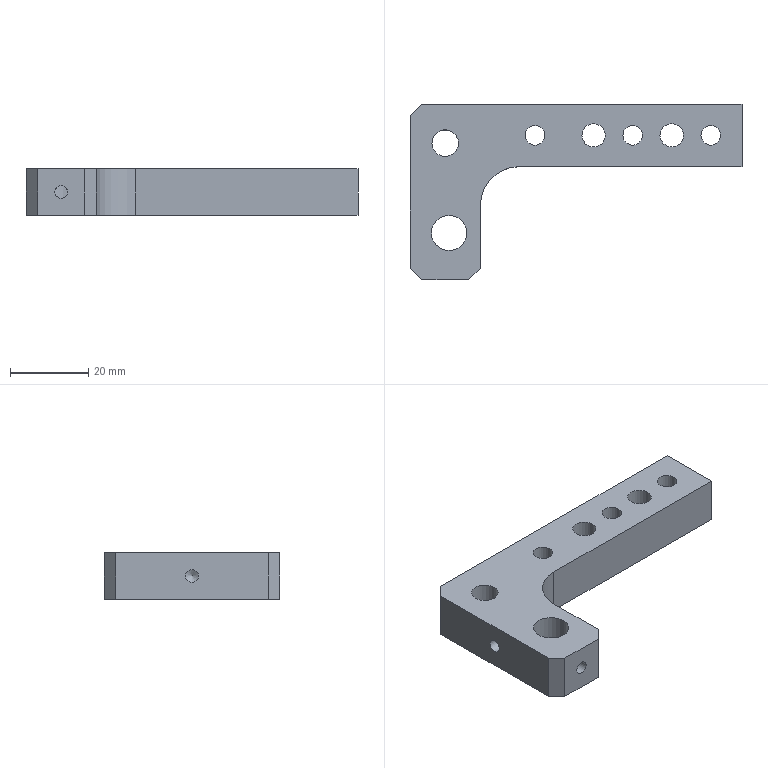Part | NX | features BREP 1 | 1 solid | 23 faces | box 85 x 45 x 12 mm | volume 19882 mm3 | plane 11 | cylinder 11 | cone 1 | commonest cylinder face diameters 3.3 x3 5 x3 6 x2 6.8 x1 9 x1 20 x1
STEP:
#1=CARTESIAN_POINT('',(-14.5,-8.,12.));
#2=VERTEX_POINT('',#1);
#3=CARTESIAN_POINT('',(42.5,-8.,12.));
#4=VERTEX_POINT('',#3);
#5=CARTESIAN_POINT('',(0.,-8.,12.));
#6=DIRECTION('',(1.,0.,0.));
#7=VECTOR('',#6,1000.);
#8=LINE('',#5,#7);
#9=EDGE_CURVE('',#2,#4,#8,.T.);
#10=ORIENTED_EDGE('',*,*,#9,.T.);
#11=CARTESIAN_POINT('',(42.5,8.,12.));
#12=VERTEX_POINT('',#11);
#13=CARTESIAN_POINT('',(42.5,0.,12.));
#14=DIRECTION('',(0.,1.,0.));
#15=VECTOR('',#14,1000.);
#16=LINE('',#13,#15);
#17=EDGE_CURVE('',#4,#12,#16,.T.);
#18=ORIENTED_EDGE('',*,*,#17,.T.);
#19=CARTESIAN_POINT('',(-39.5,8.,12.));
#20=VERTEX_POINT('',#19);
#21=CARTESIAN_POINT('',(0.,8.,12.));
#22=DIRECTION('',(-1.,0.,0.));
#23=VECTOR('',#22,1000.);
#24=LINE('',#21,#23);
#25=EDGE_CURVE('',#12,#20,#24,.T.);
#26=ORIENTED_EDGE('',*,*,#25,.T.);
#27=CARTESIAN_POINT('',(-42.5,5.,12.));
#28=VERTEX_POINT('',#27);
#29=CARTESIAN_POINT('',(-39.5,8.,12.));
#30=DIRECTION('',(-0.7071,-0.7071,0.));
#31=VECTOR('',#30,1000.);
#32=LINE('',#29,#31);
#33=EDGE_CURVE('',#20,#28,#32,.T.);
#34=ORIENTED_EDGE('',*,*,#33,.T.);
#35=CARTESIAN_POINT('',(-42.5,-34.,12.));
#36=VERTEX_POINT('',#35);
#37=CARTESIAN_POINT('',(-42.5,0.,12.));
#38=DIRECTION('',(0.,-1.,0.));
#39=VECTOR('',#38,1000.);
#40=LINE('',#37,#39);
#41=EDGE_CURVE('',#28,#36,#40,.T.);
#42=ORIENTED_EDGE('',*,*,#41,.T.);
#43=CARTESIAN_POINT('',(-39.5,-37.,12.));
#44=VERTEX_POINT('',#43);
#45=CARTESIAN_POINT('',(-42.5,-34.,12.));
#46=DIRECTION('',(0.7071,-0.7071,0.));
#47=VECTOR('',#46,1000.);
#48=LINE('',#45,#47);
#49=EDGE_CURVE('',#36,#44,#48,.T.);
#50=ORIENTED_EDGE('',*,*,#49,.T.);
#51=CARTESIAN_POINT('',(-27.5,-37.,12.));
#52=VERTEX_POINT('',#51);
#53=CARTESIAN_POINT('',(0.,-37.,12.));
#54=DIRECTION('',(1.,0.,0.));
#55=VECTOR('',#54,1000.);
#56=LINE('',#53,#55);
#57=EDGE_CURVE('',#44,#52,#56,.T.);
#58=ORIENTED_EDGE('',*,*,#57,.T.);
#59=CARTESIAN_POINT('',(-24.5,-34.,12.));
#60=VERTEX_POINT('',#59);
#61=CARTESIAN_POINT('',(-27.5,-37.,12.));
#62=DIRECTION('',(0.7071,0.7071,0.));
#63=VECTOR('',#62,1000.);
#64=LINE('',#61,#63);
#65=EDGE_CURVE('',#52,#60,#64,.T.);
#66=ORIENTED_EDGE('',*,*,#65,.T.);
#67=CARTESIAN_POINT('',(-24.5,-18.,12.));
#68=VERTEX_POINT('',#67);
#69=CARTESIAN_POINT('',(-24.5,0.,12.));
#70=DIRECTION('',(0.,1.,0.));
#71=VECTOR('',#70,1000.);
#72=LINE('',#69,#71);
#73=EDGE_CURVE('',#60,#68,#72,.T.);
#74=ORIENTED_EDGE('',*,*,#73,.T.);
#75=CARTESIAN_POINT('',(-14.5,-18.,12.));
#76=DIRECTION('',(0.,0.,-1.));
#77=DIRECTION('',(1.,0.,0.));
#78=AXIS2_PLACEMENT_3D('',#75,#76,#77);
#79=CIRCLE('',#78,10.);
#80=EDGE_CURVE('',#68,#2,#79,.T.);
#81=ORIENTED_EDGE('',*,*,#80,.T.);
#82=EDGE_LOOP('',(#10,#18,#26,#34,#42,#50,#58,#66,#74,#81));
#83=FACE_BOUND('',#82,.T.);
#84=CARTESIAN_POINT('',(-28.,-25.,12.));
#85=VERTEX_POINT('',#84);
#86=CARTESIAN_POINT('',(-32.5,-25.,12.));
#87=DIRECTION('',(0.,0.,-1.));
#88=DIRECTION('',(1.,0.,0.));
#89=AXIS2_PLACEMENT_3D('',#86,#87,#88);
#90=CIRCLE('',#89,4.5);
#91=EDGE_CURVE('',#85,#85,#90,.T.);
#92=ORIENTED_EDGE('',*,*,#91,.T.);
#93=EDGE_LOOP('',(#92));
#94=FACE_BOUND('',#93,.T.);
#95=CARTESIAN_POINT('',(12.,0.,12.));
#96=VERTEX_POINT('',#95);
#97=CARTESIAN_POINT('',(14.5,0.,12.));
#98=DIRECTION('',(0.,0.,-1.));
#99=DIRECTION('',(-1.,0.,0.));
#100=AXIS2_PLACEMENT_3D('',#97,#98,#99);
#101=CIRCLE('',#100,2.5);
#102=EDGE_CURVE('',#96,#96,#101,.T.);
#103=ORIENTED_EDGE('',*,*,#102,.T.);
#104=EDGE_LOOP('',(#103));
#105=FACE_BOUND('',#104,.T.);
#106=CARTESIAN_POINT('',(32.,0.,12.));
#107=VERTEX_POINT('',#106);
#108=CARTESIAN_POINT('',(34.5,0.,12.));
#109=DIRECTION('',(0.,0.,-1.));
#110=DIRECTION('',(-1.,0.,0.));
#111=AXIS2_PLACEMENT_3D('',#108,#109,#110);
#112=CIRCLE('',#111,2.5);
#113=EDGE_CURVE('',#107,#107,#112,.T.);
#114=ORIENTED_EDGE('',*,*,#113,.T.);
#115=EDGE_LOOP('',(#114));
#116=FACE_BOUND('',#115,.T.);
#117=CARTESIAN_POINT('',(1.5,0.,12.));
#118=VERTEX_POINT('',#117);
#119=CARTESIAN_POINT('',(4.5,0.,12.));
#120=DIRECTION('',(0.,0.,-1.));
#121=DIRECTION('',(-1.,0.,0.));
#122=AXIS2_PLACEMENT_3D('',#119,#120,#121);
#123=CIRCLE('',#122,3.);
#124=EDGE_CURVE('',#118,#118,#123,.T.);
#125=ORIENTED_EDGE('',*,*,#124,.T.);
#126=EDGE_LOOP('',(#125));
#127=FACE_BOUND('',#126,.T.);
#128=CARTESIAN_POINT('',(21.5,0.,12.));
#129=VERTEX_POINT('',#128);
#130=CARTESIAN_POINT('',(24.5,0.,12.));
#131=DIRECTION('',(0.,0.,-1.));
#132=DIRECTION('',(-1.,0.,0.));
#133=AXIS2_PLACEMENT_3D('',#130,#131,#132);
#134=CIRCLE('',#133,3.);
#135=EDGE_CURVE('',#129,#129,#134,.T.);
#136=ORIENTED_EDGE('',*,*,#135,.T.);
#137=EDGE_LOOP('',(#136));
#138=FACE_BOUND('',#137,.T.);
#139=CARTESIAN_POINT('',(-30.1,-2.,12.));
#140=VERTEX_POINT('',#139);
#141=CARTESIAN_POINT('',(-33.5,-2.,12.));
#142=DIRECTION('',(0.,0.,-1.));
#143=DIRECTION('',(1.,0.,0.));
#144=AXIS2_PLACEMENT_3D('',#141,#142,#143);
#145=CIRCLE('',#144,3.4);
#146=EDGE_CURVE('',#140,#140,#145,.T.);
#147=ORIENTED_EDGE('',*,*,#146,.T.);
#148=EDGE_LOOP('',(#147));
#149=FACE_BOUND('',#148,.T.);
#150=CARTESIAN_POINT('',(-13.,0.,12.));
#151=VERTEX_POINT('',#150);
#152=CARTESIAN_POINT('',(-10.5,0.,12.));
#153=DIRECTION('',(0.,0.,-1.));
#154=DIRECTION('',(-1.,0.,0.));
#155=AXIS2_PLACEMENT_3D('',#152,#153,#154);
#156=CIRCLE('',#155,2.5);
#157=EDGE_CURVE('',#151,#151,#156,.T.);
#158=ORIENTED_EDGE('',*,*,#157,.T.);
#159=EDGE_LOOP('',(#158));
#160=FACE_BOUND('',#159,.T.);
#161=CARTESIAN_POINT('',(0.,0.,12.));
#162=DIRECTION('',(0.,0.,1.));
#163=DIRECTION('',(-1.,0.,0.));
#164=AXIS2_PLACEMENT_3D('',#161,#162,#163);
#165=PLANE('',#164);
#166=ADVANCED_FACE('',(#83,#94,#105,#116,#127,#138,#149,#160),#165,.T.);
#167=CARTESIAN_POINT('',(42.5,8.,0.));
#168=VERTEX_POINT('',#167);
#169=CARTESIAN_POINT('',(42.5,8.,12.));
#170=DIRECTION('',(0.,0.,-1.));
#171=VECTOR('',#170,1000.);
#172=LINE('',#169,#171);
#173=EDGE_CURVE('',#12,#168,#172,.T.);
#174=ORIENTED_EDGE('',*,*,#173,.F.);
#175=ORIENTED_EDGE('',*,*,#17,.F.);
#176=CARTESIAN_POINT('',(42.5,-8.,0.));
#177=VERTEX_POINT('',#176);
#178=CARTESIAN_POINT('',(42.5,-8.,12.));
#179=DIRECTION('',(0.,0.,1.));
#180=VECTOR('',#179,1000.);
#181=LINE('',#178,#180);
#182=EDGE_CURVE('',#177,#4,#181,.T.);
#183=ORIENTED_EDGE('',*,*,#182,.F.);
#184=CARTESIAN_POINT('',(42.5,8.,0.));
#185=DIRECTION('',(0.,-1.,0.));
#186=VECTOR('',#185,1000.);
#187=LINE('',#184,#186);
#188=EDGE_CURVE('',#168,#177,#187,.T.);
#189=ORIENTED_EDGE('',*,*,#188,.F.);
#190=EDGE_LOOP('',(#174,#175,#183,#189));
#191=FACE_BOUND('',#190,.T.);
#192=CARTESIAN_POINT('',(42.5,8.,12.));
#193=DIRECTION('',(-1.,0.,0.));
#194=DIRECTION('',(0.,0.,-1.));
#195=AXIS2_PLACEMENT_3D('',#192,#193,#194);
#196=PLANE('',#195);
#197=ADVANCED_FACE('',(#191),#196,.F.);
#198=CARTESIAN_POINT('',(-14.5,-8.,0.));
#199=VERTEX_POINT('',#198);
#200=CARTESIAN_POINT('',(-14.5,-8.,12.));
#201=DIRECTION('',(0.,0.,1.));
#202=VECTOR('',#201,1000.);
#203=LINE('',#200,#202);
#204=EDGE_CURVE('',#199,#2,#203,.T.);
#205=ORIENTED_EDGE('',*,*,#204,.F.);
#206=CARTESIAN_POINT('',(-42.5,-8.,0.));
#207=DIRECTION('',(-1.,0.,0.));
#208=VECTOR('',#207,1000.);
#209=LINE('',#206,#208);
#210=EDGE_CURVE('',#177,#199,#209,.T.);
#211=ORIENTED_EDGE('',*,*,#210,.F.);
#212=ORIENTED_EDGE('',*,*,#182,.T.);
#213=ORIENTED_EDGE('',*,*,#9,.F.);
#214=EDGE_LOOP('',(#205,#211,#212,#213));
#215=FACE_BOUND('',#214,.T.);
#216=CARTESIAN_POINT('',(-42.5,-8.,12.));
#217=DIRECTION('',(0.,1.,0.));
#218=DIRECTION('',(0.,0.,-1.));
#219=AXIS2_PLACEMENT_3D('',#216,#217,#218);
#220=PLANE('',#219);
#221=ADVANCED_FACE('',(#215),#220,.F.);
#222=ORIENTED_EDGE('',*,*,#204,.T.);
#223=ORIENTED_EDGE('',*,*,#80,.F.);
#224=CARTESIAN_POINT('',(-24.5,-18.,0.));
#225=VERTEX_POINT('',#224);
#226=CARTESIAN_POINT('',(-24.5,-18.,0.));
#227=DIRECTION('',(0.,0.,1.));
#228=VECTOR('',#227,1000.);
#229=LINE('',#226,#228);
#230=EDGE_CURVE('',#225,#68,#229,.T.);
#231=ORIENTED_EDGE('',*,*,#230,.F.);
#232=CARTESIAN_POINT('',(-14.5,-18.,0.));
#233=DIRECTION('',(0.,0.,1.));
#234=DIRECTION('',(1.,0.,0.));
#235=AXIS2_PLACEMENT_3D('',#232,#233,#234);
#236=CIRCLE('',#235,10.);
#237=EDGE_CURVE('',#199,#225,#236,.T.);
#238=ORIENTED_EDGE('',*,*,#237,.F.);
#239=EDGE_LOOP('',(#222,#223,#231,#238));
#240=FACE_BOUND('',#239,.T.);
#241=CARTESIAN_POINT('',(-14.5,-18.,0.));
#242=DIRECTION('',(0.,0.,1.));
#243=DIRECTION('',(-1.,0.,0.));
#244=AXIS2_PLACEMENT_3D('',#241,#242,#243);
#245=CYLINDRICAL_SURFACE('',#244,10.);
#246=ADVANCED_FACE('',(#240),#245,.F.);
#247=CARTESIAN_POINT('',(-24.5,-34.,0.));
#248=VERTEX_POINT('',#247);
#249=CARTESIAN_POINT('',(-24.5,-8.,0.));
#250=DIRECTION('',(0.,1.,0.));
#251=VECTOR('',#250,1000.);
#252=LINE('',#249,#251);
#253=EDGE_CURVE('',#248,#225,#252,.T.);
#254=ORIENTED_EDGE('',*,*,#253,.T.);
#255=ORIENTED_EDGE('',*,*,#230,.T.);
#256=ORIENTED_EDGE('',*,*,#73,.F.);
#257=CARTESIAN_POINT('',(-24.5,-34.,0.));
#258=DIRECTION('',(0.,0.,-1.));
#259=VECTOR('',#258,1000.);
#260=LINE('',#257,#259);
#261=EDGE_CURVE('',#60,#248,#260,.T.);
#262=ORIENTED_EDGE('',*,*,#261,.T.);
#263=EDGE_LOOP('',(#254,#255,#256,#262));
#264=FACE_BOUND('',#263,.T.);
#265=CARTESIAN_POINT('',(-24.5,-8.,0.));
#266=DIRECTION('',(1.,0.,0.));
#267=DIRECTION('',(0.,-1.,0.));
#268=AXIS2_PLACEMENT_3D('',#265,#266,#267);
#269=PLANE('',#268);
#270=ADVANCED_FACE('',(#264),#269,.T.);
#271=ORIENTED_EDGE('',*,*,#261,.F.);
#272=ORIENTED_EDGE('',*,*,#65,.F.);
#273=CARTESIAN_POINT('',(-27.5,-37.,0.));
#274=VERTEX_POINT('',#273);
#275=CARTESIAN_POINT('',(-27.5,-37.,0.));
#276=DIRECTION('',(0.,0.,1.));
#277=VECTOR('',#276,1000.);
#278=LINE('',#275,#277);
#279=EDGE_CURVE('',#274,#52,#278,.T.);
#280=ORIENTED_EDGE('',*,*,#279,.F.);
#281=CARTESIAN_POINT('',(-27.5,-37.,0.));
#282=DIRECTION('',(-0.7071,-0.7071,0.));
#283=VECTOR('',#282,1000.);
#284=LINE('',#281,#283);
#285=EDGE_CURVE('',#248,#274,#284,.T.);
#286=ORIENTED_EDGE('',*,*,#285,.F.);
#287=EDGE_LOOP('',(#271,#272,#280,#286));
#288=FACE_BOUND('',#287,.T.);
#289=CARTESIAN_POINT('',(-27.5,-37.,0.));
#290=DIRECTION('',(-0.7071,0.7071,0.));
#291=DIRECTION('',(0.7071,0.7071,0.));
#292=AXIS2_PLACEMENT_3D('',#289,#290,#291);
#293=PLANE('',#292);
#294=ADVANCED_FACE('',(#288),#293,.F.);
#295=CARTESIAN_POINT('',(-39.5,-37.,0.));
#296=VERTEX_POINT('',#295);
#297=CARTESIAN_POINT('',(-24.5,-37.,0.));
#298=DIRECTION('',(1.,0.,0.));
#299=VECTOR('',#298,1000.);
#300=LINE('',#297,#299);
#301=EDGE_CURVE('',#296,#274,#300,.T.);
#302=ORIENTED_EDGE('',*,*,#301,.T.);
#303=ORIENTED_EDGE('',*,*,#279,.T.);
#304=ORIENTED_EDGE('',*,*,#57,.F.);
#305=CARTESIAN_POINT('',(-39.5,-37.,0.));
#306=DIRECTION('',(0.,0.,-1.));
#307=VECTOR('',#306,1000.);
#308=LINE('',#305,#307);
#309=EDGE_CURVE('',#44,#296,#308,.T.);
#310=ORIENTED_EDGE('',*,*,#309,.T.);
#311=EDGE_LOOP('',(#302,#303,#304,#310));
#312=FACE_BOUND('',#311,.T.);
#313=CARTESIAN_POINT('',(-33.5,-37.,4.35));
#314=VERTEX_POINT('',#313);
#315=CARTESIAN_POINT('',(-33.5,-37.,6.));
#316=DIRECTION('',(0.,1.,0.));
#317=DIRECTION('',(0.,0.,-1.));
#318=AXIS2_PLACEMENT_3D('',#315,#316,#317);
#319=CIRCLE('',#318,1.65);
#320=EDGE_CURVE('',#314,#314,#319,.T.);
#321=ORIENTED_EDGE('',*,*,#320,.T.);
#322=EDGE_LOOP('',(#321));
#323=FACE_BOUND('',#322,.T.);
#324=CARTESIAN_POINT('',(-24.5,-37.,0.));
#325=DIRECTION('',(0.,-1.,0.));
#326=DIRECTION('',(-1.,0.,0.));
#327=AXIS2_PLACEMENT_3D('',#324,#325,#326);
#328=PLANE('',#327);
#329=ADVANCED_FACE('',(#312,#323),#328,.T.);
#330=ORIENTED_EDGE('',*,*,#49,.F.);
#331=CARTESIAN_POINT('',(-42.5,-34.,0.));
#332=VERTEX_POINT('',#331);
#333=CARTESIAN_POINT('',(-42.5,-34.,12.));
#334=DIRECTION('',(0.,0.,-1.));
#335=VECTOR('',#334,1000.);
#336=LINE('',#333,#335);
#337=EDGE_CURVE('',#36,#332,#336,.T.);
#338=ORIENTED_EDGE('',*,*,#337,.T.);
#339=CARTESIAN_POINT('',(-42.5,-34.,0.));
#340=DIRECTION('',(0.7071,-0.7071,0.));
#341=VECTOR('',#340,1000.);
#342=LINE('',#339,#341);
#343=EDGE_CURVE('',#332,#296,#342,.T.);
#344=ORIENTED_EDGE('',*,*,#343,.T.);
#345=ORIENTED_EDGE('',*,*,#309,.F.);
#346=EDGE_LOOP('',(#330,#338,#344,#345));
#347=FACE_BOUND('',#346,.T.);
#348=CARTESIAN_POINT('',(-42.5,-34.,12.));
#349=DIRECTION('',(-0.7071,-0.7071,0.));
#350=DIRECTION('',(-0.7071,0.7071,0.));
#351=AXIS2_PLACEMENT_3D('',#348,#349,#350);
#352=PLANE('',#351);
#353=ADVANCED_FACE('',(#347),#352,.T.);
#354=CARTESIAN_POINT('',(-42.5,5.,0.));
#355=VERTEX_POINT('',#354);
#356=CARTESIAN_POINT('',(-42.5,5.,12.));
#357=DIRECTION('',(0.,0.,1.));
#358=VECTOR('',#357,1000.);
#359=LINE('',#356,#358);
#360=EDGE_CURVE('',#355,#28,#359,.T.);
#361=ORIENTED_EDGE('',*,*,#360,.F.);
#362=CARTESIAN_POINT('',(-42.5,8.,0.));
#363=DIRECTION('',(0.,1.,0.));
#364=VECTOR('',#363,1000.);
#365=LINE('',#362,#364);
#366=EDGE_CURVE('',#332,#355,#365,.T.);
#367=ORIENTED_EDGE('',*,*,#366,.F.);
#368=ORIENTED_EDGE('',*,*,#337,.F.);
#369=ORIENTED_EDGE('',*,*,#41,.F.);
#370=EDGE_LOOP('',(#361,#367,#368,#369));
#371=FACE_BOUND('',#370,.T.);
#372=CARTESIAN_POINT('',(-42.5,-14.5,7.65));
#373=VERTEX_POINT('',#372);
#374=CARTESIAN_POINT('',(-42.5,-14.5,6.));
#375=DIRECTION('',(-1.,0.,0.));
#376=DIRECTION('',(0.,0.,1.));
#377=AXIS2_PLACEMENT_3D('',#374,#375,#376);
#378=CIRCLE('',#377,1.65);
#379=EDGE_CURVE('',#373,#373,#378,.T.);
#380=ORIENTED_EDGE('',*,*,#379,.F.);
#381=EDGE_LOOP('',(#380));
#382=FACE_BOUND('',#381,.T.);
#383=CARTESIAN_POINT('',(-42.5,8.,12.));
#384=DIRECTION('',(1.,0.,0.));
#385=DIRECTION('',(0.,0.,1.));
#386=AXIS2_PLACEMENT_3D('',#383,#384,#385);
#387=PLANE('',#386);
#388=ADVANCED_FACE('',(#371,#382),#387,.F.);
#389=CARTESIAN_POINT('',(-39.5,8.,0.));
#390=VERTEX_POINT('',#389);
#391=CARTESIAN_POINT('',(-39.5,8.,12.));
#392=DIRECTION('',(0.,0.,1.));
#393=VECTOR('',#392,1000.);
#394=LINE('',#391,#393);
#395=EDGE_CURVE('',#390,#20,#394,.T.);
#396=ORIENTED_EDGE('',*,*,#395,.F.);
#397=CARTESIAN_POINT('',(-42.5,5.,0.));
#398=DIRECTION('',(0.7071,0.7071,0.));
#399=VECTOR('',#398,1000.);
#400=LINE('',#397,#399);
#401=EDGE_CURVE('',#355,#390,#400,.T.);
#402=ORIENTED_EDGE('',*,*,#401,.F.);
#403=ORIENTED_EDGE('',*,*,#360,.T.);
#404=ORIENTED_EDGE('',*,*,#33,.F.);
#405=EDGE_LOOP('',(#396,#402,#403,#404));
#406=FACE_BOUND('',#405,.T.);
#407=CARTESIAN_POINT('',(-42.5,5.,12.));
#408=DIRECTION('',(0.7071,-0.7071,0.));
#409=DIRECTION('',(-0.7071,-0.7071,0.));
#410=AXIS2_PLACEMENT_3D('',#407,#408,#409);
#411=PLANE('',#410);
#412=ADVANCED_FACE('',(#406),#411,.F.);
#413=ORIENTED_EDGE('',*,*,#395,.T.);
#414=ORIENTED_EDGE('',*,*,#25,.F.);
#415=ORIENTED_EDGE('',*,*,#173,.T.);
#416=CARTESIAN_POINT('',(-42.5,8.,0.));
#417=DIRECTION('',(1.,0.,0.));
#418=VECTOR('',#417,1000.);
#419=LINE('',#416,#418);
#420=EDGE_CURVE('',#390,#168,#419,.T.);
#421=ORIENTED_EDGE('',*,*,#420,.F.);
#422=EDGE_LOOP('',(#413,#414,#415,#421));
#423=FACE_BOUND('',#422,.T.);
#424=CARTESIAN_POINT('',(-33.5,8.,7.65));
#425=VERTEX_POINT('',#424);
#426=CARTESIAN_POINT('',(-33.5,8.,6.));
#427=DIRECTION('',(0.,1.,0.));
#428=DIRECTION('',(0.,0.,1.));
#429=AXIS2_PLACEMENT_3D('',#426,#427,#428);
#430=CIRCLE('',#429,1.65);
#431=EDGE_CURVE('',#425,#425,#430,.T.);
#432=ORIENTED_EDGE('',*,*,#431,.F.);
#433=EDGE_LOOP('',(#432));
#434=FACE_BOUND('',#433,.T.);
#435=CARTESIAN_POINT('',(-42.5,8.,12.));
#436=DIRECTION('',(0.,-1.,0.));
#437=DIRECTION('',(0.,0.,1.));
#438=AXIS2_PLACEMENT_3D('',#435,#436,#437);
#439=PLANE('',#438);
#440=ADVANCED_FACE('',(#423,#434),#439,.F.);
#441=ORIENTED_EDGE('',*,*,#91,.F.);
#442=EDGE_LOOP('',(#441));
#443=FACE_BOUND('',#442,.T.);
#444=CARTESIAN_POINT('',(-28.,-25.,0.));
#445=VERTEX_POINT('',#444);
#446=CARTESIAN_POINT('',(-32.5,-25.,0.));
#447=DIRECTION('',(0.,0.,1.));
#448=DIRECTION('',(1.,0.,0.));
#449=AXIS2_PLACEMENT_3D('',#446,#447,#448);
#450=CIRCLE('',#449,4.5);
#451=EDGE_CURVE('',#445,#445,#450,.T.);
#452=ORIENTED_EDGE('',*,*,#451,.F.);
#453=EDGE_LOOP('',(#452));
#454=FACE_BOUND('',#453,.T.);
#455=CARTESIAN_POINT('',(-33.5,-29.387,7.65));
#456=VERTEX_POINT('',#455);
#457=CARTESIAN_POINT('',(-34.745,-28.95,7.321));
#458=CARTESIAN_POINT('',(-33.519,-29.462,7.824));
#459=CARTESIAN_POINT('',(-32.179,-29.525,7.284));
#460=CARTESIAN_POINT('',(-31.665,-29.414,5.941));
#461=CARTESIAN_POINT('',(-32.268,-29.536,4.631));
#462=CARTESIAN_POINT('',(-33.634,-29.435,4.183));
#463=CARTESIAN_POINT('',(-34.821,-28.899,4.755));
#464=CARTESIAN_POINT('',(-35.332,-28.494,6.058));
#465=CARTESIAN_POINT('',(-34.745,-28.95,7.321));
#466=CARTESIAN_POINT('',(-33.519,-29.462,7.824));
#467=CARTESIAN_POINT('',(-32.179,-29.525,7.284));
#468=B_SPLINE_CURVE_WITH_KNOTS('',3,(#457,#458,#459,#460,#461,#462,#463,#464,#465,#466,#467),.UNSPECIFIED.,.T.,.F.,(1,1,1,1,1,1,1,1,1,1,1,1,1,1,1),(-0.003964,-0.002643,-0.001321,0.,0.001321,0.002643,0.003964,0.005285,0.006606,0.007928,0.009249,0.01057,0.01189,0.01321,0.01453),.UNSPECIFIED.);
#469=EDGE_CURVE('',#456,#456,#468,.T.);
#470=ORIENTED_EDGE('',*,*,#469,.F.);
#471=EDGE_LOOP('',(#470));
#472=FACE_BOUND('',#471,.T.);
#473=CARTESIAN_POINT('',(-32.5,-25.,12.));
#474=DIRECTION('',(0.,0.,1.));
#475=DIRECTION('',(-1.,0.,0.));
#476=AXIS2_PLACEMENT_3D('',#473,#474,#475);
#477=CYLINDRICAL_SURFACE('',#476,4.5);
#478=ADVANCED_FACE('',(#443,#454,#472),#477,.F.);
#479=CARTESIAN_POINT('',(12.,0.,0.));
#480=VERTEX_POINT('',#479);
#481=CARTESIAN_POINT('',(14.5,0.,0.));
#482=DIRECTION('',(0.,0.,1.));
#483=DIRECTION('',(-1.,0.,0.));
#484=AXIS2_PLACEMENT_3D('',#481,#482,#483);
#485=CIRCLE('',#484,2.5);
#486=EDGE_CURVE('',#480,#480,#485,.T.);
#487=ORIENTED_EDGE('',*,*,#486,.F.);
#488=EDGE_LOOP('',(#487));
#489=FACE_BOUND('',#488,.T.);
#490=ORIENTED_EDGE('',*,*,#102,.F.);
#491=EDGE_LOOP('',(#490));
#492=FACE_BOUND('',#491,.T.);
#493=CARTESIAN_POINT('',(14.5,0.,0.));
#494=DIRECTION('',(0.,0.,-1.));
#495=DIRECTION('',(1.,0.,0.));
#496=AXIS2_PLACEMENT_3D('',#493,#494,#495);
#497=CYLINDRICAL_SURFACE('',#496,2.5);
#498=ADVANCED_FACE('',(#489,#492),#497,.F.);
#499=CARTESIAN_POINT('',(32.,0.,0.));
#500=VERTEX_POINT('',#499);
#501=CARTESIAN_POINT('',(34.5,0.,0.));
#502=DIRECTION('',(0.,0.,1.));
#503=DIRECTION('',(-1.,0.,0.));
#504=AXIS2_PLACEMENT_3D('',#501,#502,#503);
#505=CIRCLE('',#504,2.5);
#506=EDGE_CURVE('',#500,#500,#505,.T.);
#507=ORIENTED_EDGE('',*,*,#506,.F.);
#508=EDGE_LOOP('',(#507));
#509=FACE_BOUND('',#508,.T.);
#510=ORIENTED_EDGE('',*,*,#113,.F.);
#511=EDGE_LOOP('',(#510));
#512=FACE_BOUND('',#511,.T.);
#513=CARTESIAN_POINT('',(34.5,0.,0.));
#514=DIRECTION('',(0.,0.,-1.));
#515=DIRECTION('',(1.,0.,0.));
#516=AXIS2_PLACEMENT_3D('',#513,#514,#515);
#517=CYLINDRICAL_SURFACE('',#516,2.5);
#518=ADVANCED_FACE('',(#509,#512),#517,.F.);
#519=CARTESIAN_POINT('',(1.5,0.,0.));
#520=VERTEX_POINT('',#519);
#521=CARTESIAN_POINT('',(4.5,0.,0.));
#522=DIRECTION('',(0.,0.,1.));
#523=DIRECTION('',(-1.,0.,0.));
#524=AXIS2_PLACEMENT_3D('',#521,#522,#523);
#525=CIRCLE('',#524,3.);
#526=EDGE_CURVE('',#520,#520,#525,.T.);
#527=ORIENTED_EDGE('',*,*,#526,.F.);
#528=EDGE_LOOP('',(#527));
#529=FACE_BOUND('',#528,.T.);
#530=ORIENTED_EDGE('',*,*,#124,.F.);
#531=EDGE_LOOP('',(#530));
#532=FACE_BOUND('',#531,.T.);
#533=CARTESIAN_POINT('',(4.5,0.,0.));
#534=DIRECTION('',(0.,0.,-1.));
#535=DIRECTION('',(1.,0.,0.));
#536=AXIS2_PLACEMENT_3D('',#533,#534,#535);
#537=CYLINDRICAL_SURFACE('',#536,3.);
#538=ADVANCED_FACE('',(#529,#532),#537,.F.);
#539=CARTESIAN_POINT('',(21.5,0.,0.));
#540=VERTEX_POINT('',#539);
#541=CARTESIAN_POINT('',(24.5,0.,0.));
#542=DIRECTION('',(0.,0.,1.));
#543=DIRECTION('',(-1.,0.,0.));
#544=AXIS2_PLACEMENT_3D('',#541,#542,#543);
#545=CIRCLE('',#544,3.);
#546=EDGE_CURVE('',#540,#540,#545,.T.);
#547=ORIENTED_EDGE('',*,*,#546,.F.);
#548=EDGE_LOOP('',(#547));
#549=FACE_BOUND('',#548,.T.);
#550=ORIENTED_EDGE('',*,*,#135,.F.);
#551=EDGE_LOOP('',(#550));
#552=FACE_BOUND('',#551,.T.);
#553=CARTESIAN_POINT('',(24.5,0.,0.));
#554=DIRECTION('',(0.,0.,-1.));
#555=DIRECTION('',(1.,0.,0.));
#556=AXIS2_PLACEMENT_3D('',#553,#554,#555);
#557=CYLINDRICAL_SURFACE('',#556,3.);
#558=ADVANCED_FACE('',(#549,#552),#557,.F.);
#559=ORIENTED_EDGE('',*,*,#146,.F.);
#560=EDGE_LOOP('',(#559));
#561=FACE_BOUND('',#560,.T.);
#562=CARTESIAN_POINT('',(-30.1,-2.,0.));
#563=VERTEX_POINT('',#562);
#564=CARTESIAN_POINT('',(-33.5,-2.,0.));
#565=DIRECTION('',(0.,0.,1.));
#566=DIRECTION('',(1.,0.,0.));
#567=AXIS2_PLACEMENT_3D('',#564,#565,#566);
#568=CIRCLE('',#567,3.4);
#569=EDGE_CURVE('',#563,#563,#568,.T.);
#570=ORIENTED_EDGE('',*,*,#569,.F.);
#571=EDGE_LOOP('',(#570));
#572=FACE_BOUND('',#571,.T.);
#573=CARTESIAN_POINT('',(-33.5,1.4,4.35));
#574=VERTEX_POINT('',#573);
#575=CARTESIAN_POINT('',(-34.796,1.2,4.708));
#576=CARTESIAN_POINT('',(-33.5,1.5,4.171));
#577=CARTESIAN_POINT('',(-32.206,1.2,4.709));
#578=CARTESIAN_POINT('',(-31.672,0.8593,5.995));
#579=CARTESIAN_POINT('',(-32.205,1.199,7.291));
#580=CARTESIAN_POINT('',(-33.494,1.5,7.829));
#581=CARTESIAN_POINT('',(-34.794,1.201,7.292));
#582=CARTESIAN_POINT('',(-35.328,0.8591,6.005));
#583=CARTESIAN_POINT('',(-34.796,1.2,4.708));
#584=CARTESIAN_POINT('',(-33.5,1.5,4.171));
#585=CARTESIAN_POINT('',(-32.206,1.2,4.709));
#586=B_SPLINE_CURVE_WITH_KNOTS('',3,(#575,#576,#577,#578,#579,#580,#581,#582,#583,#584,#585),.UNSPECIFIED.,.T.,.F.,(1,1,1,1,1,1,1,1,1,1,1,1,1,1,1),(-0.003929,-0.002619,-0.00131,0.,0.00131,0.002619,0.003929,0.005239,0.006548,0.007858,0.009168,0.01048,0.01179,0.0131,0.01441),.UNSPECIFIED.);
#587=EDGE_CURVE('',#574,#574,#586,.T.);
#588=ORIENTED_EDGE('',*,*,#587,.F.);
#589=EDGE_LOOP('',(#588));
#590=FACE_BOUND('',#589,.T.);
#591=CARTESIAN_POINT('',(-33.5,-2.,12.));
#592=DIRECTION('',(0.,0.,1.));
#593=DIRECTION('',(-1.,0.,0.));
#594=AXIS2_PLACEMENT_3D('',#591,#592,#593);
#595=CYLINDRICAL_SURFACE('',#594,3.4);
#596=ADVANCED_FACE('',(#561,#572,#590),#595,.F.);
#597=CARTESIAN_POINT('',(-13.,0.,0.));
#598=VERTEX_POINT('',#597);
#599=CARTESIAN_POINT('',(-10.5,0.,0.));
#600=DIRECTION('',(0.,0.,1.));
#601=DIRECTION('',(-1.,0.,0.));
#602=AXIS2_PLACEMENT_3D('',#599,#600,#601);
#603=CIRCLE('',#602,2.5);
#604=EDGE_CURVE('',#598,#598,#603,.T.);
#605=ORIENTED_EDGE('',*,*,#604,.F.);
#606=EDGE_LOOP('',(#605));
#607=FACE_BOUND('',#606,.T.);
#608=ORIENTED_EDGE('',*,*,#157,.F.);
#609=EDGE_LOOP('',(#608));
#610=FACE_BOUND('',#609,.T.);
#611=CARTESIAN_POINT('',(-10.5,0.,0.));
#612=DIRECTION('',(0.,0.,-1.));
#613=DIRECTION('',(1.,0.,0.));
#614=AXIS2_PLACEMENT_3D('',#611,#612,#613);
#615=CYLINDRICAL_SURFACE('',#614,2.5);
#616=ADVANCED_FACE('',(#607,#610),#615,.F.);
#617=ORIENTED_EDGE('',*,*,#604,.T.);
#618=EDGE_LOOP('',(#617));
#619=FACE_BOUND('',#618,.T.);
#620=ORIENTED_EDGE('',*,*,#401,.T.);
#621=ORIENTED_EDGE('',*,*,#420,.T.);
#622=ORIENTED_EDGE('',*,*,#188,.T.);
#623=ORIENTED_EDGE('',*,*,#210,.T.);
#624=ORIENTED_EDGE('',*,*,#237,.T.);
#625=ORIENTED_EDGE('',*,*,#253,.F.);
#626=ORIENTED_EDGE('',*,*,#285,.T.);
#627=ORIENTED_EDGE('',*,*,#301,.F.);
#628=ORIENTED_EDGE('',*,*,#343,.F.);
#629=ORIENTED_EDGE('',*,*,#366,.T.);
#630=EDGE_LOOP('',(#620,#621,#622,#623,#624,#625,#626,#627,#628,#629));
#631=FACE_BOUND('',#630,.T.);
#632=ORIENTED_EDGE('',*,*,#451,.T.);
#633=EDGE_LOOP('',(#632));
#634=FACE_BOUND('',#633,.T.);
#635=ORIENTED_EDGE('',*,*,#486,.T.);
#636=EDGE_LOOP('',(#635));
#637=FACE_BOUND('',#636,.T.);
#638=ORIENTED_EDGE('',*,*,#506,.T.);
#639=EDGE_LOOP('',(#638));
#640=FACE_BOUND('',#639,.T.);
#641=ORIENTED_EDGE('',*,*,#526,.T.);
#642=EDGE_LOOP('',(#641));
#643=FACE_BOUND('',#642,.T.);
#644=ORIENTED_EDGE('',*,*,#546,.T.);
#645=EDGE_LOOP('',(#644));
#646=FACE_BOUND('',#645,.T.);
#647=ORIENTED_EDGE('',*,*,#569,.T.);
#648=EDGE_LOOP('',(#647));
#649=FACE_BOUND('',#648,.T.);
#650=CARTESIAN_POINT('',(0.,0.,0.));
#651=DIRECTION('',(0.,0.,1.));
#652=DIRECTION('',(-1.,0.,0.));
#653=AXIS2_PLACEMENT_3D('',#650,#651,#652);
#654=PLANE('',#653);
#655=ADVANCED_FACE('',(#619,#631,#634,#637,#640,#643,#646,#649),#654,.F.);
#656=ORIENTED_EDGE('',*,*,#320,.F.);
#657=EDGE_LOOP('',(#656));
#658=FACE_BOUND('',#657,.T.);
#659=ORIENTED_EDGE('',*,*,#469,.T.);
#660=EDGE_LOOP('',(#659));
#661=FACE_BOUND('',#660,.T.);
#662=CARTESIAN_POINT('',(-33.5,-37.,6.));
#663=DIRECTION('',(0.,-1.,0.));
#664=DIRECTION('',(0.,0.,1.));
#665=AXIS2_PLACEMENT_3D('',#662,#663,#664);
#666=CYLINDRICAL_SURFACE('',#665,1.65);
#667=ADVANCED_FACE('',(#658,#661),#666,.F.);
#668=CARTESIAN_POINT('',(-32.4,-14.5,7.65));
#669=VERTEX_POINT('',#668);
#670=CARTESIAN_POINT('',(-32.4,-14.5,6.));
#671=DIRECTION('',(-1.,0.,0.));
#672=DIRECTION('',(0.,0.,1.));
#673=AXIS2_PLACEMENT_3D('',#670,#671,#672);
#674=CIRCLE('',#673,1.65);
#675=EDGE_CURVE('',#669,#669,#674,.T.);
#676=ORIENTED_EDGE('',*,*,#675,.F.);
#677=EDGE_LOOP('',(#676));
#678=FACE_BOUND('',#677,.T.);
#679=ORIENTED_EDGE('',*,*,#379,.T.);
#680=EDGE_LOOP('',(#679));
#681=FACE_BOUND('',#680,.T.);
#682=CARTESIAN_POINT('',(-42.5,-14.5,6.));
#683=DIRECTION('',(-1.,0.,0.));
#684=DIRECTION('',(0.,0.,-1.));
#685=AXIS2_PLACEMENT_3D('',#682,#683,#684);
#686=CYLINDRICAL_SURFACE('',#685,1.65);
#687=ADVANCED_FACE('',(#678,#681),#686,.F.);
#688=ORIENTED_EDGE('',*,*,#587,.T.);
#689=EDGE_LOOP('',(#688));
#690=FACE_BOUND('',#689,.T.);
#691=ORIENTED_EDGE('',*,*,#431,.T.);
#692=EDGE_LOOP('',(#691));
#693=FACE_BOUND('',#692,.T.);
#694=CARTESIAN_POINT('',(-33.5,8.,6.));
#695=DIRECTION('',(0.,1.,0.));
#696=DIRECTION('',(0.,0.,-1.));
#697=AXIS2_PLACEMENT_3D('',#694,#695,#696);
#698=CYLINDRICAL_SURFACE('',#697,1.65);
#699=ADVANCED_FACE('',(#690,#693),#698,.F.);
#700=CARTESIAN_POINT('',(-31.409,-14.5,6.));
#701=VERTEX_POINT('',#700);
#702=VERTEX_LOOP('',#701);
#703=FACE_BOUND('',#702,.T.);
#704=ORIENTED_EDGE('',*,*,#675,.T.);
#705=EDGE_LOOP('',(#704));
#706=FACE_BOUND('',#705,.T.);
#707=CARTESIAN_POINT('',(-32.4,-14.5,6.));
#708=DIRECTION('',(-1.,0.,0.));
#709=DIRECTION('',(0.,0.,-1.));
#710=AXIS2_PLACEMENT_3D('',#707,#708,#709);
#711=CONICAL_SURFACE('',#710,1.65,1.03);
#712=ADVANCED_FACE('',(#703,#706),#711,.F.);
#713=CLOSED_SHELL('',(#166,#197,#221,#246,#270,#294,#329,#353,#388,#412,#440,#478,#498,#518,#538,#558,#596,#616,#655,#667,#687,#699,#712));
#714=MANIFOLD_SOLID_BREP('',#713);
#715=(LENGTH_UNIT()NAMED_UNIT(*)SI_UNIT(.MILLI.,.METRE.));
#716=UNCERTAINTY_MEASURE_WITH_UNIT(LENGTH_MEASURE(0.0508),#715,'','');
#717=(NAMED_UNIT(*)PLANE_ANGLE_UNIT()SI_UNIT($,.RADIAN.));
#718=(NAMED_UNIT(*)SI_UNIT($,.STERADIAN.)SOLID_ANGLE_UNIT());
#719=(GEOMETRIC_REPRESENTATION_CONTEXT(3)GLOBAL_UNCERTAINTY_ASSIGNED_CONTEXT((#716))GLOBAL_UNIT_ASSIGNED_CONTEXT((#715,#717,#718))REPRESENTATION_CONTEXT('',''));
#720=ADVANCED_BREP_SHAPE_REPRESENTATION('',(#714),#719);